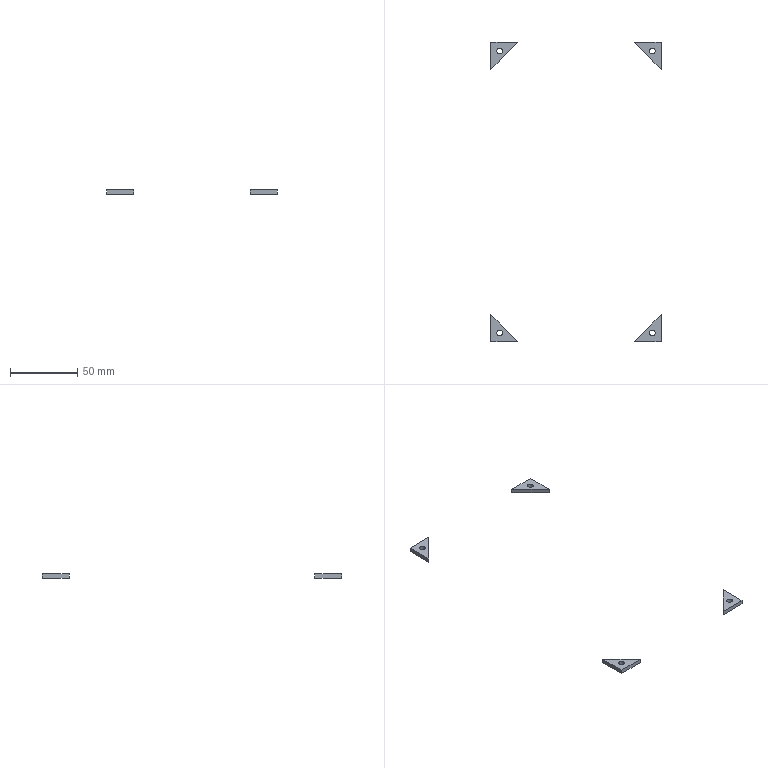Part | NX | features DATUM_CSYS 1, EXTRACT_DATUM_PLANE 1, EXTRUDE 1, SKETCH 1 | 4 solids | 24 faces | box 127 x 223 x 3 mm | volume 2234 mm3 | plane 20 | cylinder 4 | commonest cylinder face diameters 4.2 x4
STEP:
#1=CARTESIAN_POINT('',(-63.5,-91.5,70.));
#2=VERTEX_POINT('',#1);
#3=CARTESIAN_POINT('',(-63.5,-111.5,70.));
#4=VERTEX_POINT('',#3);
#5=CARTESIAN_POINT('',(-63.5,-91.5,70.));
#6=DIRECTION('',(0.,-1.,0.));
#7=VECTOR('',#6,1000.);
#8=LINE('',#5,#7);
#9=EDGE_CURVE('',#2,#4,#8,.T.);
#10=ORIENTED_EDGE('',*,*,#9,.F.);
#11=CARTESIAN_POINT('',(-63.5,-91.5,67.));
#12=VERTEX_POINT('',#11);
#13=CARTESIAN_POINT('',(-63.5,-91.5,67.));
#14=DIRECTION('',(0.,0.,1.));
#15=VECTOR('',#14,1000.);
#16=LINE('',#13,#15);
#17=EDGE_CURVE('',#12,#2,#16,.T.);
#18=ORIENTED_EDGE('',*,*,#17,.F.);
#19=CARTESIAN_POINT('',(-63.5,-111.5,67.));
#20=VERTEX_POINT('',#19);
#21=CARTESIAN_POINT('',(-63.5,-91.5,67.));
#22=DIRECTION('',(0.,-1.,0.));
#23=VECTOR('',#22,1000.);
#24=LINE('',#21,#23);
#25=EDGE_CURVE('',#12,#20,#24,.T.);
#26=ORIENTED_EDGE('',*,*,#25,.T.);
#27=CARTESIAN_POINT('',(-63.5,-111.5,67.));
#28=DIRECTION('',(0.,0.,1.));
#29=VECTOR('',#28,1000.);
#30=LINE('',#27,#29);
#31=EDGE_CURVE('',#20,#4,#30,.T.);
#32=ORIENTED_EDGE('',*,*,#31,.T.);
#33=EDGE_LOOP('',(#10,#18,#26,#32));
#34=FACE_BOUND('',#33,.T.);
#35=CARTESIAN_POINT('',(-63.5,-91.5,67.));
#36=DIRECTION('',(-1.,0.,0.));
#37=DIRECTION('',(0.,0.,1.));
#38=AXIS2_PLACEMENT_3D('',#35,#36,#37);
#39=PLANE('',#38);
#40=ADVANCED_FACE('',(#34),#39,.T.);
#41=CARTESIAN_POINT('',(-43.5,-111.5,70.));
#42=VERTEX_POINT('',#41);
#43=CARTESIAN_POINT('',(-63.5,-111.5,70.));
#44=DIRECTION('',(1.,0.,0.));
#45=VECTOR('',#44,1000.);
#46=LINE('',#43,#45);
#47=EDGE_CURVE('',#4,#42,#46,.T.);
#48=ORIENTED_EDGE('',*,*,#47,.F.);
#49=ORIENTED_EDGE('',*,*,#31,.F.);
#50=CARTESIAN_POINT('',(-43.5,-111.5,67.));
#51=VERTEX_POINT('',#50);
#52=CARTESIAN_POINT('',(-63.5,-111.5,67.));
#53=DIRECTION('',(1.,0.,0.));
#54=VECTOR('',#53,1000.);
#55=LINE('',#52,#54);
#56=EDGE_CURVE('',#20,#51,#55,.T.);
#57=ORIENTED_EDGE('',*,*,#56,.T.);
#58=CARTESIAN_POINT('',(-43.5,-111.5,67.));
#59=DIRECTION('',(0.,0.,1.));
#60=VECTOR('',#59,1000.);
#61=LINE('',#58,#60);
#62=EDGE_CURVE('',#51,#42,#61,.T.);
#63=ORIENTED_EDGE('',*,*,#62,.T.);
#64=EDGE_LOOP('',(#48,#49,#57,#63));
#65=FACE_BOUND('',#64,.T.);
#66=CARTESIAN_POINT('',(-63.5,-111.5,67.));
#67=DIRECTION('',(0.,-1.,0.));
#68=DIRECTION('',(0.,0.,-1.));
#69=AXIS2_PLACEMENT_3D('',#66,#67,#68);
#70=PLANE('',#69);
#71=ADVANCED_FACE('',(#65),#70,.T.);
#72=CARTESIAN_POINT('',(-43.5,-111.5,70.));
#73=DIRECTION('',(-0.7071,0.7071,0.));
#74=VECTOR('',#73,1000.);
#75=LINE('',#72,#74);
#76=EDGE_CURVE('',#42,#2,#75,.T.);
#77=ORIENTED_EDGE('',*,*,#76,.F.);
#78=ORIENTED_EDGE('',*,*,#62,.F.);
#79=CARTESIAN_POINT('',(-43.5,-111.5,67.));
#80=DIRECTION('',(-0.7071,0.7071,0.));
#81=VECTOR('',#80,1000.);
#82=LINE('',#79,#81);
#83=EDGE_CURVE('',#51,#12,#82,.T.);
#84=ORIENTED_EDGE('',*,*,#83,.T.);
#85=ORIENTED_EDGE('',*,*,#17,.T.);
#86=EDGE_LOOP('',(#77,#78,#84,#85));
#87=FACE_BOUND('',#86,.T.);
#88=CARTESIAN_POINT('',(-43.5,-111.5,67.));
#89=DIRECTION('',(0.7071,0.7071,0.));
#90=DIRECTION('',(-0.7071,0.7071,0.));
#91=AXIS2_PLACEMENT_3D('',#88,#89,#90);
#92=PLANE('',#91);
#93=ADVANCED_FACE('',(#87),#92,.T.);
#94=CARTESIAN_POINT('',(-59.1,-105.,70.));
#95=VERTEX_POINT('',#94);
#96=CARTESIAN_POINT('',(-57.,-105.,70.));
#97=DIRECTION('',(0.,0.,-1.));
#98=DIRECTION('',(-1.,0.,0.));
#99=AXIS2_PLACEMENT_3D('',#96,#97,#98);
#100=CIRCLE('',#99,2.1);
#101=EDGE_CURVE('',#95,#95,#100,.T.);
#102=ORIENTED_EDGE('',*,*,#101,.F.);
#103=EDGE_LOOP('',(#102));
#104=FACE_BOUND('',#103,.T.);
#105=CARTESIAN_POINT('',(-54.9,-105.,67.));
#106=VERTEX_POINT('',#105);
#107=CARTESIAN_POINT('',(-57.,-105.,67.));
#108=DIRECTION('',(0.,0.,-1.));
#109=DIRECTION('',(1.,0.,0.));
#110=AXIS2_PLACEMENT_3D('',#107,#108,#109);
#111=CIRCLE('',#110,2.1);
#112=EDGE_CURVE('',#106,#106,#111,.T.);
#113=ORIENTED_EDGE('',*,*,#112,.T.);
#114=EDGE_LOOP('',(#113));
#115=FACE_BOUND('',#114,.T.);
#116=CARTESIAN_POINT('',(-57.,-105.,67.));
#117=DIRECTION('',(0.,0.,1.));
#118=DIRECTION('',(1.,0.,0.));
#119=AXIS2_PLACEMENT_3D('',#116,#117,#118);
#120=CYLINDRICAL_SURFACE('',#119,2.1);
#121=ADVANCED_FACE('',(#104,#115),#120,.F.);
#122=ORIENTED_EDGE('',*,*,#25,.F.);
#123=ORIENTED_EDGE('',*,*,#83,.F.);
#124=ORIENTED_EDGE('',*,*,#56,.F.);
#125=EDGE_LOOP('',(#122,#123,#124));
#126=FACE_BOUND('',#125,.T.);
#127=ORIENTED_EDGE('',*,*,#112,.F.);
#128=EDGE_LOOP('',(#127));
#129=FACE_BOUND('',#128,.T.);
#130=CARTESIAN_POINT('',(-57.,-105.,67.));
#131=DIRECTION('',(0.,0.,-1.));
#132=DIRECTION('',(-1.,0.,0.));
#133=AXIS2_PLACEMENT_3D('',#130,#131,#132);
#134=PLANE('',#133);
#135=ADVANCED_FACE('',(#126,#129),#134,.T.);
#136=ORIENTED_EDGE('',*,*,#9,.T.);
#137=ORIENTED_EDGE('',*,*,#47,.T.);
#138=ORIENTED_EDGE('',*,*,#76,.T.);
#139=EDGE_LOOP('',(#136,#137,#138));
#140=FACE_BOUND('',#139,.T.);
#141=ORIENTED_EDGE('',*,*,#101,.T.);
#142=EDGE_LOOP('',(#141));
#143=FACE_BOUND('',#142,.T.);
#144=CARTESIAN_POINT('',(-57.,-105.,70.));
#145=DIRECTION('',(0.,0.,-1.));
#146=DIRECTION('',(-1.,0.,0.));
#147=AXIS2_PLACEMENT_3D('',#144,#145,#146);
#148=PLANE('',#147);
#149=ADVANCED_FACE('',(#140,#143),#148,.F.);
#150=CLOSED_SHELL('',(#40,#71,#93,#121,#135,#149));
#151=MANIFOLD_SOLID_BREP('',#150);
#152=CARTESIAN_POINT('',(43.5,111.5,70.));
#153=VERTEX_POINT('',#152);
#154=CARTESIAN_POINT('',(63.5,91.5,70.));
#155=VERTEX_POINT('',#154);
#156=CARTESIAN_POINT('',(43.5,111.5,70.));
#157=DIRECTION('',(0.7071,-0.7071,0.));
#158=VECTOR('',#157,1000.);
#159=LINE('',#156,#158);
#160=EDGE_CURVE('',#153,#155,#159,.T.);
#161=ORIENTED_EDGE('',*,*,#160,.F.);
#162=CARTESIAN_POINT('',(43.5,111.5,67.));
#163=VERTEX_POINT('',#162);
#164=CARTESIAN_POINT('',(43.5,111.5,67.));
#165=DIRECTION('',(0.,0.,1.));
#166=VECTOR('',#165,1000.);
#167=LINE('',#164,#166);
#168=EDGE_CURVE('',#163,#153,#167,.T.);
#169=ORIENTED_EDGE('',*,*,#168,.F.);
#170=CARTESIAN_POINT('',(63.5,91.5,67.));
#171=VERTEX_POINT('',#170);
#172=CARTESIAN_POINT('',(43.5,111.5,67.));
#173=DIRECTION('',(0.7071,-0.7071,0.));
#174=VECTOR('',#173,1000.);
#175=LINE('',#172,#174);
#176=EDGE_CURVE('',#163,#171,#175,.T.);
#177=ORIENTED_EDGE('',*,*,#176,.T.);
#178=CARTESIAN_POINT('',(63.5,91.5,67.));
#179=DIRECTION('',(0.,0.,1.));
#180=VECTOR('',#179,1000.);
#181=LINE('',#178,#180);
#182=EDGE_CURVE('',#171,#155,#181,.T.);
#183=ORIENTED_EDGE('',*,*,#182,.T.);
#184=EDGE_LOOP('',(#161,#169,#177,#183));
#185=FACE_BOUND('',#184,.T.);
#186=CARTESIAN_POINT('',(43.5,111.5,67.));
#187=DIRECTION('',(-0.7071,-0.7071,0.));
#188=DIRECTION('',(0.7071,-0.7071,0.));
#189=AXIS2_PLACEMENT_3D('',#186,#187,#188);
#190=PLANE('',#189);
#191=ADVANCED_FACE('',(#185),#190,.T.);
#192=CARTESIAN_POINT('',(63.5,111.5,70.));
#193=VERTEX_POINT('',#192);
#194=CARTESIAN_POINT('',(63.5,91.5,70.));
#195=DIRECTION('',(0.,1.,0.));
#196=VECTOR('',#195,1000.);
#197=LINE('',#194,#196);
#198=EDGE_CURVE('',#155,#193,#197,.T.);
#199=ORIENTED_EDGE('',*,*,#198,.F.);
#200=ORIENTED_EDGE('',*,*,#182,.F.);
#201=CARTESIAN_POINT('',(63.5,111.5,67.));
#202=VERTEX_POINT('',#201);
#203=CARTESIAN_POINT('',(63.5,91.5,67.));
#204=DIRECTION('',(0.,1.,0.));
#205=VECTOR('',#204,1000.);
#206=LINE('',#203,#205);
#207=EDGE_CURVE('',#171,#202,#206,.T.);
#208=ORIENTED_EDGE('',*,*,#207,.T.);
#209=CARTESIAN_POINT('',(63.5,111.5,67.));
#210=DIRECTION('',(0.,0.,1.));
#211=VECTOR('',#210,1000.);
#212=LINE('',#209,#211);
#213=EDGE_CURVE('',#202,#193,#212,.T.);
#214=ORIENTED_EDGE('',*,*,#213,.T.);
#215=EDGE_LOOP('',(#199,#200,#208,#214));
#216=FACE_BOUND('',#215,.T.);
#217=CARTESIAN_POINT('',(63.5,91.5,67.));
#218=DIRECTION('',(1.,0.,0.));
#219=DIRECTION('',(0.,0.,-1.));
#220=AXIS2_PLACEMENT_3D('',#217,#218,#219);
#221=PLANE('',#220);
#222=ADVANCED_FACE('',(#216),#221,.T.);
#223=CARTESIAN_POINT('',(63.5,111.5,70.));
#224=DIRECTION('',(-1.,0.,0.));
#225=VECTOR('',#224,1000.);
#226=LINE('',#223,#225);
#227=EDGE_CURVE('',#193,#153,#226,.T.);
#228=ORIENTED_EDGE('',*,*,#227,.F.);
#229=ORIENTED_EDGE('',*,*,#213,.F.);
#230=CARTESIAN_POINT('',(63.5,111.5,67.));
#231=DIRECTION('',(-1.,0.,0.));
#232=VECTOR('',#231,1000.);
#233=LINE('',#230,#232);
#234=EDGE_CURVE('',#202,#163,#233,.T.);
#235=ORIENTED_EDGE('',*,*,#234,.T.);
#236=ORIENTED_EDGE('',*,*,#168,.T.);
#237=EDGE_LOOP('',(#228,#229,#235,#236));
#238=FACE_BOUND('',#237,.T.);
#239=CARTESIAN_POINT('',(63.5,111.5,67.));
#240=DIRECTION('',(0.,1.,0.));
#241=DIRECTION('',(0.,0.,1.));
#242=AXIS2_PLACEMENT_3D('',#239,#240,#241);
#243=PLANE('',#242);
#244=ADVANCED_FACE('',(#238),#243,.T.);
#245=CARTESIAN_POINT('',(54.9,105.,70.));
#246=VERTEX_POINT('',#245);
#247=CARTESIAN_POINT('',(57.,105.,70.));
#248=DIRECTION('',(0.,0.,-1.));
#249=DIRECTION('',(-1.,0.,0.));
#250=AXIS2_PLACEMENT_3D('',#247,#248,#249);
#251=CIRCLE('',#250,2.1);
#252=EDGE_CURVE('',#246,#246,#251,.T.);
#253=ORIENTED_EDGE('',*,*,#252,.F.);
#254=EDGE_LOOP('',(#253));
#255=FACE_BOUND('',#254,.T.);
#256=CARTESIAN_POINT('',(59.1,105.,67.));
#257=VERTEX_POINT('',#256);
#258=CARTESIAN_POINT('',(57.,105.,67.));
#259=DIRECTION('',(0.,0.,-1.));
#260=DIRECTION('',(1.,0.,0.));
#261=AXIS2_PLACEMENT_3D('',#258,#259,#260);
#262=CIRCLE('',#261,2.1);
#263=EDGE_CURVE('',#257,#257,#262,.T.);
#264=ORIENTED_EDGE('',*,*,#263,.T.);
#265=EDGE_LOOP('',(#264));
#266=FACE_BOUND('',#265,.T.);
#267=CARTESIAN_POINT('',(57.,105.,67.));
#268=DIRECTION('',(0.,0.,1.));
#269=DIRECTION('',(1.,0.,0.));
#270=AXIS2_PLACEMENT_3D('',#267,#268,#269);
#271=CYLINDRICAL_SURFACE('',#270,2.1);
#272=ADVANCED_FACE('',(#255,#266),#271,.F.);
#273=ORIENTED_EDGE('',*,*,#176,.F.);
#274=ORIENTED_EDGE('',*,*,#234,.F.);
#275=ORIENTED_EDGE('',*,*,#207,.F.);
#276=EDGE_LOOP('',(#273,#274,#275));
#277=FACE_BOUND('',#276,.T.);
#278=ORIENTED_EDGE('',*,*,#263,.F.);
#279=EDGE_LOOP('',(#278));
#280=FACE_BOUND('',#279,.T.);
#281=CARTESIAN_POINT('',(57.,105.,67.));
#282=DIRECTION('',(0.,0.,-1.));
#283=DIRECTION('',(-1.,0.,0.));
#284=AXIS2_PLACEMENT_3D('',#281,#282,#283);
#285=PLANE('',#284);
#286=ADVANCED_FACE('',(#277,#280),#285,.T.);
#287=ORIENTED_EDGE('',*,*,#160,.T.);
#288=ORIENTED_EDGE('',*,*,#198,.T.);
#289=ORIENTED_EDGE('',*,*,#227,.T.);
#290=EDGE_LOOP('',(#287,#288,#289));
#291=FACE_BOUND('',#290,.T.);
#292=ORIENTED_EDGE('',*,*,#252,.T.);
#293=EDGE_LOOP('',(#292));
#294=FACE_BOUND('',#293,.T.);
#295=CARTESIAN_POINT('',(57.,105.,70.));
#296=DIRECTION('',(0.,0.,-1.));
#297=DIRECTION('',(-1.,0.,0.));
#298=AXIS2_PLACEMENT_3D('',#295,#296,#297);
#299=PLANE('',#298);
#300=ADVANCED_FACE('',(#291,#294),#299,.F.);
#301=CLOSED_SHELL('',(#191,#222,#244,#272,#286,#300));
#302=MANIFOLD_SOLID_BREP('',#301);
#303=CARTESIAN_POINT('',(-63.5,111.5,70.));
#304=VERTEX_POINT('',#303);
#305=CARTESIAN_POINT('',(-63.5,91.5,70.));
#306=VERTEX_POINT('',#305);
#307=CARTESIAN_POINT('',(-63.5,111.5,70.));
#308=DIRECTION('',(0.,-1.,0.));
#309=VECTOR('',#308,1000.);
#310=LINE('',#307,#309);
#311=EDGE_CURVE('',#304,#306,#310,.T.);
#312=ORIENTED_EDGE('',*,*,#311,.F.);
#313=CARTESIAN_POINT('',(-63.5,111.5,67.));
#314=VERTEX_POINT('',#313);
#315=CARTESIAN_POINT('',(-63.5,111.5,67.));
#316=DIRECTION('',(0.,0.,1.));
#317=VECTOR('',#316,1000.);
#318=LINE('',#315,#317);
#319=EDGE_CURVE('',#314,#304,#318,.T.);
#320=ORIENTED_EDGE('',*,*,#319,.F.);
#321=CARTESIAN_POINT('',(-63.5,91.5,67.));
#322=VERTEX_POINT('',#321);
#323=CARTESIAN_POINT('',(-63.5,111.5,67.));
#324=DIRECTION('',(0.,-1.,0.));
#325=VECTOR('',#324,1000.);
#326=LINE('',#323,#325);
#327=EDGE_CURVE('',#314,#322,#326,.T.);
#328=ORIENTED_EDGE('',*,*,#327,.T.);
#329=CARTESIAN_POINT('',(-63.5,91.5,67.));
#330=DIRECTION('',(0.,0.,1.));
#331=VECTOR('',#330,1000.);
#332=LINE('',#329,#331);
#333=EDGE_CURVE('',#322,#306,#332,.T.);
#334=ORIENTED_EDGE('',*,*,#333,.T.);
#335=EDGE_LOOP('',(#312,#320,#328,#334));
#336=FACE_BOUND('',#335,.T.);
#337=CARTESIAN_POINT('',(-63.5,111.5,67.));
#338=DIRECTION('',(-1.,0.,0.));
#339=DIRECTION('',(0.,0.,1.));
#340=AXIS2_PLACEMENT_3D('',#337,#338,#339);
#341=PLANE('',#340);
#342=ADVANCED_FACE('',(#336),#341,.T.);
#343=CARTESIAN_POINT('',(-43.5,111.5,70.));
#344=VERTEX_POINT('',#343);
#345=CARTESIAN_POINT('',(-63.5,91.5,70.));
#346=DIRECTION('',(0.7071,0.7071,0.));
#347=VECTOR('',#346,1000.);
#348=LINE('',#345,#347);
#349=EDGE_CURVE('',#306,#344,#348,.T.);
#350=ORIENTED_EDGE('',*,*,#349,.F.);
#351=ORIENTED_EDGE('',*,*,#333,.F.);
#352=CARTESIAN_POINT('',(-43.5,111.5,67.));
#353=VERTEX_POINT('',#352);
#354=CARTESIAN_POINT('',(-63.5,91.5,67.));
#355=DIRECTION('',(0.7071,0.7071,0.));
#356=VECTOR('',#355,1000.);
#357=LINE('',#354,#356);
#358=EDGE_CURVE('',#322,#353,#357,.T.);
#359=ORIENTED_EDGE('',*,*,#358,.T.);
#360=CARTESIAN_POINT('',(-43.5,111.5,67.));
#361=DIRECTION('',(0.,0.,1.));
#362=VECTOR('',#361,1000.);
#363=LINE('',#360,#362);
#364=EDGE_CURVE('',#353,#344,#363,.T.);
#365=ORIENTED_EDGE('',*,*,#364,.T.);
#366=EDGE_LOOP('',(#350,#351,#359,#365));
#367=FACE_BOUND('',#366,.T.);
#368=CARTESIAN_POINT('',(-63.5,91.5,67.));
#369=DIRECTION('',(0.7071,-0.7071,0.));
#370=DIRECTION('',(0.7071,0.7071,0.));
#371=AXIS2_PLACEMENT_3D('',#368,#369,#370);
#372=PLANE('',#371);
#373=ADVANCED_FACE('',(#367),#372,.T.);
#374=CARTESIAN_POINT('',(-43.5,111.5,70.));
#375=DIRECTION('',(-1.,0.,0.));
#376=VECTOR('',#375,1000.);
#377=LINE('',#374,#376);
#378=EDGE_CURVE('',#344,#304,#377,.T.);
#379=ORIENTED_EDGE('',*,*,#378,.F.);
#380=ORIENTED_EDGE('',*,*,#364,.F.);
#381=CARTESIAN_POINT('',(-43.5,111.5,67.));
#382=DIRECTION('',(-1.,0.,0.));
#383=VECTOR('',#382,1000.);
#384=LINE('',#381,#383);
#385=EDGE_CURVE('',#353,#314,#384,.T.);
#386=ORIENTED_EDGE('',*,*,#385,.T.);
#387=ORIENTED_EDGE('',*,*,#319,.T.);
#388=EDGE_LOOP('',(#379,#380,#386,#387));
#389=FACE_BOUND('',#388,.T.);
#390=CARTESIAN_POINT('',(-43.5,111.5,67.));
#391=DIRECTION('',(0.,1.,0.));
#392=DIRECTION('',(0.,0.,1.));
#393=AXIS2_PLACEMENT_3D('',#390,#391,#392);
#394=PLANE('',#393);
#395=ADVANCED_FACE('',(#389),#394,.T.);
#396=CARTESIAN_POINT('',(-59.1,105.,70.));
#397=VERTEX_POINT('',#396);
#398=CARTESIAN_POINT('',(-57.,105.,70.));
#399=DIRECTION('',(0.,0.,-1.));
#400=DIRECTION('',(-1.,0.,0.));
#401=AXIS2_PLACEMENT_3D('',#398,#399,#400);
#402=CIRCLE('',#401,2.1);
#403=EDGE_CURVE('',#397,#397,#402,.T.);
#404=ORIENTED_EDGE('',*,*,#403,.F.);
#405=EDGE_LOOP('',(#404));
#406=FACE_BOUND('',#405,.T.);
#407=CARTESIAN_POINT('',(-54.9,105.,67.));
#408=VERTEX_POINT('',#407);
#409=CARTESIAN_POINT('',(-57.,105.,67.));
#410=DIRECTION('',(0.,0.,-1.));
#411=DIRECTION('',(1.,0.,0.));
#412=AXIS2_PLACEMENT_3D('',#409,#410,#411);
#413=CIRCLE('',#412,2.1);
#414=EDGE_CURVE('',#408,#408,#413,.T.);
#415=ORIENTED_EDGE('',*,*,#414,.T.);
#416=EDGE_LOOP('',(#415));
#417=FACE_BOUND('',#416,.T.);
#418=CARTESIAN_POINT('',(-57.,105.,67.));
#419=DIRECTION('',(0.,0.,1.));
#420=DIRECTION('',(1.,0.,0.));
#421=AXIS2_PLACEMENT_3D('',#418,#419,#420);
#422=CYLINDRICAL_SURFACE('',#421,2.1);
#423=ADVANCED_FACE('',(#406,#417),#422,.F.);
#424=ORIENTED_EDGE('',*,*,#327,.F.);
#425=ORIENTED_EDGE('',*,*,#385,.F.);
#426=ORIENTED_EDGE('',*,*,#358,.F.);
#427=EDGE_LOOP('',(#424,#425,#426));
#428=FACE_BOUND('',#427,.T.);
#429=ORIENTED_EDGE('',*,*,#414,.F.);
#430=EDGE_LOOP('',(#429));
#431=FACE_BOUND('',#430,.T.);
#432=CARTESIAN_POINT('',(-57.,105.,67.));
#433=DIRECTION('',(0.,0.,-1.));
#434=DIRECTION('',(-1.,0.,0.));
#435=AXIS2_PLACEMENT_3D('',#432,#433,#434);
#436=PLANE('',#435);
#437=ADVANCED_FACE('',(#428,#431),#436,.T.);
#438=ORIENTED_EDGE('',*,*,#311,.T.);
#439=ORIENTED_EDGE('',*,*,#349,.T.);
#440=ORIENTED_EDGE('',*,*,#378,.T.);
#441=EDGE_LOOP('',(#438,#439,#440));
#442=FACE_BOUND('',#441,.T.);
#443=ORIENTED_EDGE('',*,*,#403,.T.);
#444=EDGE_LOOP('',(#443));
#445=FACE_BOUND('',#444,.T.);
#446=CARTESIAN_POINT('',(-57.,105.,70.));
#447=DIRECTION('',(0.,0.,-1.));
#448=DIRECTION('',(-1.,0.,0.));
#449=AXIS2_PLACEMENT_3D('',#446,#447,#448);
#450=PLANE('',#449);
#451=ADVANCED_FACE('',(#442,#445),#450,.F.);
#452=CLOSED_SHELL('',(#342,#373,#395,#423,#437,#451));
#453=MANIFOLD_SOLID_BREP('',#452);
#454=CARTESIAN_POINT('',(43.5,-111.5,70.));
#455=VERTEX_POINT('',#454);
#456=CARTESIAN_POINT('',(63.5,-111.5,70.));
#457=VERTEX_POINT('',#456);
#458=CARTESIAN_POINT('',(43.5,-111.5,70.));
#459=DIRECTION('',(1.,0.,0.));
#460=VECTOR('',#459,1000.);
#461=LINE('',#458,#460);
#462=EDGE_CURVE('',#455,#457,#461,.T.);
#463=ORIENTED_EDGE('',*,*,#462,.F.);
#464=CARTESIAN_POINT('',(43.5,-111.5,67.));
#465=VERTEX_POINT('',#464);
#466=CARTESIAN_POINT('',(43.5,-111.5,67.));
#467=DIRECTION('',(0.,0.,1.));
#468=VECTOR('',#467,1000.);
#469=LINE('',#466,#468);
#470=EDGE_CURVE('',#465,#455,#469,.T.);
#471=ORIENTED_EDGE('',*,*,#470,.F.);
#472=CARTESIAN_POINT('',(63.5,-111.5,67.));
#473=VERTEX_POINT('',#472);
#474=CARTESIAN_POINT('',(43.5,-111.5,67.));
#475=DIRECTION('',(1.,0.,0.));
#476=VECTOR('',#475,1000.);
#477=LINE('',#474,#476);
#478=EDGE_CURVE('',#465,#473,#477,.T.);
#479=ORIENTED_EDGE('',*,*,#478,.T.);
#480=CARTESIAN_POINT('',(63.5,-111.5,67.));
#481=DIRECTION('',(0.,0.,1.));
#482=VECTOR('',#481,1000.);
#483=LINE('',#480,#482);
#484=EDGE_CURVE('',#473,#457,#483,.T.);
#485=ORIENTED_EDGE('',*,*,#484,.T.);
#486=EDGE_LOOP('',(#463,#471,#479,#485));
#487=FACE_BOUND('',#486,.T.);
#488=CARTESIAN_POINT('',(43.5,-111.5,67.));
#489=DIRECTION('',(0.,-1.,0.));
#490=DIRECTION('',(0.,0.,-1.));
#491=AXIS2_PLACEMENT_3D('',#488,#489,#490);
#492=PLANE('',#491);
#493=ADVANCED_FACE('',(#487),#492,.T.);
#494=CARTESIAN_POINT('',(63.5,-91.5,70.));
#495=VERTEX_POINT('',#494);
#496=CARTESIAN_POINT('',(63.5,-111.5,70.));
#497=DIRECTION('',(0.,1.,0.));
#498=VECTOR('',#497,1000.);
#499=LINE('',#496,#498);
#500=EDGE_CURVE('',#457,#495,#499,.T.);
#501=ORIENTED_EDGE('',*,*,#500,.F.);
#502=ORIENTED_EDGE('',*,*,#484,.F.);
#503=CARTESIAN_POINT('',(63.5,-91.5,67.));
#504=VERTEX_POINT('',#503);
#505=CARTESIAN_POINT('',(63.5,-111.5,67.));
#506=DIRECTION('',(0.,1.,0.));
#507=VECTOR('',#506,1000.);
#508=LINE('',#505,#507);
#509=EDGE_CURVE('',#473,#504,#508,.T.);
#510=ORIENTED_EDGE('',*,*,#509,.T.);
#511=CARTESIAN_POINT('',(63.5,-91.5,67.));
#512=DIRECTION('',(0.,0.,1.));
#513=VECTOR('',#512,1000.);
#514=LINE('',#511,#513);
#515=EDGE_CURVE('',#504,#495,#514,.T.);
#516=ORIENTED_EDGE('',*,*,#515,.T.);
#517=EDGE_LOOP('',(#501,#502,#510,#516));
#518=FACE_BOUND('',#517,.T.);
#519=CARTESIAN_POINT('',(63.5,-111.5,67.));
#520=DIRECTION('',(1.,0.,0.));
#521=DIRECTION('',(0.,0.,-1.));
#522=AXIS2_PLACEMENT_3D('',#519,#520,#521);
#523=PLANE('',#522);
#524=ADVANCED_FACE('',(#518),#523,.T.);
#525=CARTESIAN_POINT('',(63.5,-91.5,70.));
#526=DIRECTION('',(-0.7071,-0.7071,0.));
#527=VECTOR('',#526,1000.);
#528=LINE('',#525,#527);
#529=EDGE_CURVE('',#495,#455,#528,.T.);
#530=ORIENTED_EDGE('',*,*,#529,.F.);
#531=ORIENTED_EDGE('',*,*,#515,.F.);
#532=CARTESIAN_POINT('',(63.5,-91.5,67.));
#533=DIRECTION('',(-0.7071,-0.7071,0.));
#534=VECTOR('',#533,1000.);
#535=LINE('',#532,#534);
#536=EDGE_CURVE('',#504,#465,#535,.T.);
#537=ORIENTED_EDGE('',*,*,#536,.T.);
#538=ORIENTED_EDGE('',*,*,#470,.T.);
#539=EDGE_LOOP('',(#530,#531,#537,#538));
#540=FACE_BOUND('',#539,.T.);
#541=CARTESIAN_POINT('',(63.5,-91.5,67.));
#542=DIRECTION('',(-0.7071,0.7071,0.));
#543=DIRECTION('',(-0.7071,-0.7071,0.));
#544=AXIS2_PLACEMENT_3D('',#541,#542,#543);
#545=PLANE('',#544);
#546=ADVANCED_FACE('',(#540),#545,.T.);
#547=CARTESIAN_POINT('',(54.9,-105.,70.));
#548=VERTEX_POINT('',#547);
#549=CARTESIAN_POINT('',(57.,-105.,70.));
#550=DIRECTION('',(0.,0.,-1.));
#551=DIRECTION('',(-1.,0.,0.));
#552=AXIS2_PLACEMENT_3D('',#549,#550,#551);
#553=CIRCLE('',#552,2.1);
#554=EDGE_CURVE('',#548,#548,#553,.T.);
#555=ORIENTED_EDGE('',*,*,#554,.F.);
#556=EDGE_LOOP('',(#555));
#557=FACE_BOUND('',#556,.T.);
#558=CARTESIAN_POINT('',(59.1,-105.,67.));
#559=VERTEX_POINT('',#558);
#560=CARTESIAN_POINT('',(57.,-105.,67.));
#561=DIRECTION('',(0.,0.,-1.));
#562=DIRECTION('',(1.,0.,0.));
#563=AXIS2_PLACEMENT_3D('',#560,#561,#562);
#564=CIRCLE('',#563,2.1);
#565=EDGE_CURVE('',#559,#559,#564,.T.);
#566=ORIENTED_EDGE('',*,*,#565,.T.);
#567=EDGE_LOOP('',(#566));
#568=FACE_BOUND('',#567,.T.);
#569=CARTESIAN_POINT('',(57.,-105.,67.));
#570=DIRECTION('',(0.,0.,1.));
#571=DIRECTION('',(1.,0.,0.));
#572=AXIS2_PLACEMENT_3D('',#569,#570,#571);
#573=CYLINDRICAL_SURFACE('',#572,2.1);
#574=ADVANCED_FACE('',(#557,#568),#573,.F.);
#575=ORIENTED_EDGE('',*,*,#478,.F.);
#576=ORIENTED_EDGE('',*,*,#536,.F.);
#577=ORIENTED_EDGE('',*,*,#509,.F.);
#578=EDGE_LOOP('',(#575,#576,#577));
#579=FACE_BOUND('',#578,.T.);
#580=ORIENTED_EDGE('',*,*,#565,.F.);
#581=EDGE_LOOP('',(#580));
#582=FACE_BOUND('',#581,.T.);
#583=CARTESIAN_POINT('',(57.,-105.,67.));
#584=DIRECTION('',(0.,0.,-1.));
#585=DIRECTION('',(-1.,0.,0.));
#586=AXIS2_PLACEMENT_3D('',#583,#584,#585);
#587=PLANE('',#586);
#588=ADVANCED_FACE('',(#579,#582),#587,.T.);
#589=ORIENTED_EDGE('',*,*,#462,.T.);
#590=ORIENTED_EDGE('',*,*,#500,.T.);
#591=ORIENTED_EDGE('',*,*,#529,.T.);
#592=EDGE_LOOP('',(#589,#590,#591));
#593=FACE_BOUND('',#592,.T.);
#594=ORIENTED_EDGE('',*,*,#554,.T.);
#595=EDGE_LOOP('',(#594));
#596=FACE_BOUND('',#595,.T.);
#597=CARTESIAN_POINT('',(57.,-105.,70.));
#598=DIRECTION('',(0.,0.,-1.));
#599=DIRECTION('',(-1.,0.,0.));
#600=AXIS2_PLACEMENT_3D('',#597,#598,#599);
#601=PLANE('',#600);
#602=ADVANCED_FACE('',(#593,#596),#601,.F.);
#603=CLOSED_SHELL('',(#493,#524,#546,#574,#588,#602));
#604=MANIFOLD_SOLID_BREP('',#603);
#605=(LENGTH_UNIT()NAMED_UNIT(*)SI_UNIT(.MILLI.,.METRE.));
#606=UNCERTAINTY_MEASURE_WITH_UNIT(LENGTH_MEASURE(0.00001),#605,'','');
#607=(NAMED_UNIT(*)PLANE_ANGLE_UNIT()SI_UNIT($,.RADIAN.));
#608=(NAMED_UNIT(*)SI_UNIT($,.STERADIAN.)SOLID_ANGLE_UNIT());
#609=(GEOMETRIC_REPRESENTATION_CONTEXT(3)GLOBAL_UNCERTAINTY_ASSIGNED_CONTEXT((#606))GLOBAL_UNIT_ASSIGNED_CONTEXT((#605,#607,#608))REPRESENTATION_CONTEXT('',''));
#610=ADVANCED_BREP_SHAPE_REPRESENTATION('',(#151,#302,#453,#604),#609);